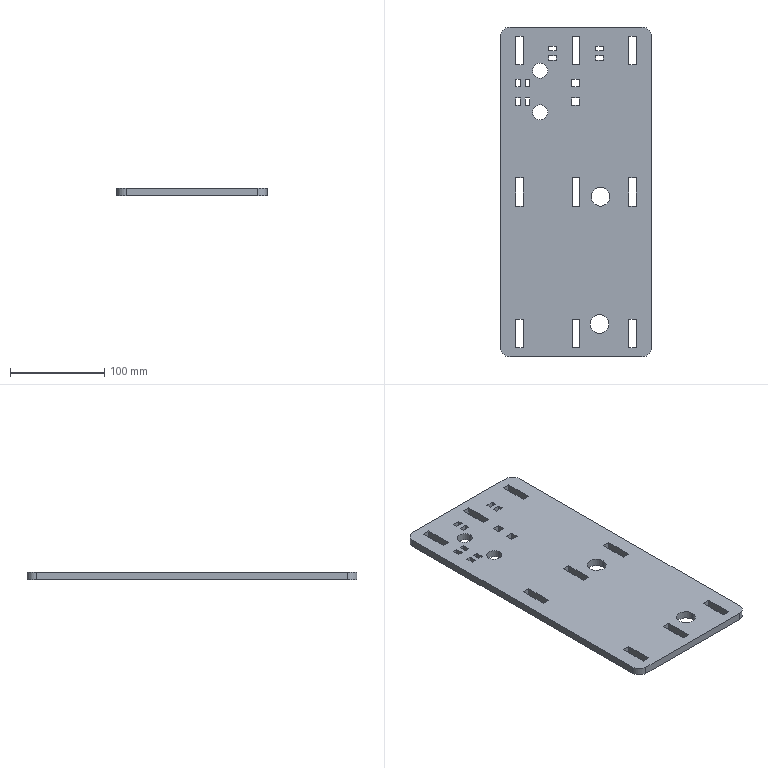Part | SolidWorks | features Fillet 1, FlatPattern 1, SMBaseFlange 1, SheetMetal 1 | 1 solid | 94 faces | box 160 x 350 x 8 mm | volume 418206 mm3 | plane 82 | cylinder 12 | commonest cylinder face diameters 20 x8 16 x4